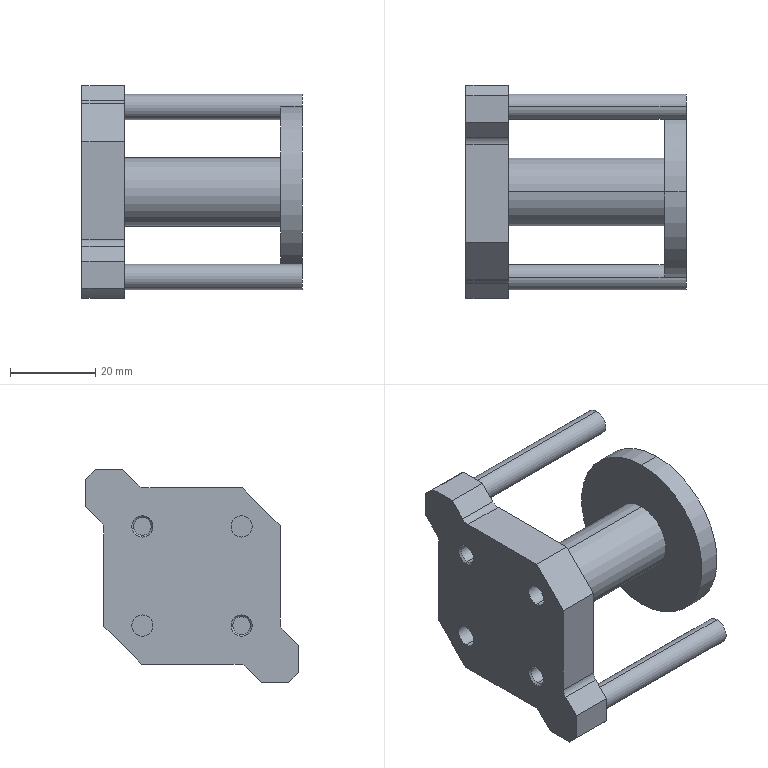Part | STEP file | 1105WWT2_1 | 1 solid | 50 faces | box 51.75 x 50 x 50 mm | volume 33168 mm3 | cylinder 22 | plane 20 | cone 8 | commonest cylinder face diameters 4.134 x4 4.6 x4 5 x4 6 x4 16 x2 40 x2
STEP:
#1=CARTESIAN_POINT('',(-7.,-11.65,9.15));
#2=VERTEX_POINT('',#1);
#3=CARTESIAN_POINT('',(-7.,-11.65,14.15));
#4=VERTEX_POINT('',#3);
#5=CARTESIAN_POINT('',(-7.,-11.65,11.65));
#6=DIRECTION('',(-1.,0.,0.));
#7=DIRECTION('',(0.,0.,1.));
#8=AXIS2_PLACEMENT_3D('',#5,#6,#7);
#9=CIRCLE('',#8,2.5);
#10=EDGE_CURVE('',#2,#4,#9,.T.);
#11=ORIENTED_EDGE('',*,*,#10,.F.);
#12=CARTESIAN_POINT('',(-17.,-11.65,9.15));
#13=VERTEX_POINT('',#12);
#14=CARTESIAN_POINT('',(-17.,-11.65,9.15));
#15=DIRECTION('',(-1.,0.,0.));
#16=VECTOR('',#15,1000.);
#17=LINE('',#14,#16);
#18=EDGE_CURVE('',#2,#13,#17,.T.);
#19=ORIENTED_EDGE('',*,*,#18,.T.);
#20=CARTESIAN_POINT('',(-17.,-11.65,14.15));
#21=VERTEX_POINT('',#20);
#22=CARTESIAN_POINT('',(-17.,-11.65,11.65));
#23=DIRECTION('',(-1.,0.,0.));
#24=DIRECTION('',(0.,0.,1.));
#25=AXIS2_PLACEMENT_3D('',#22,#23,#24);
#26=CIRCLE('',#25,2.5);
#27=EDGE_CURVE('',#13,#21,#26,.T.);
#28=ORIENTED_EDGE('',*,*,#27,.T.);
#29=CARTESIAN_POINT('',(-17.,-11.65,14.15));
#30=DIRECTION('',(-1.,0.,0.));
#31=VECTOR('',#30,1000.);
#32=LINE('',#29,#31);
#33=EDGE_CURVE('',#4,#21,#32,.T.);
#34=ORIENTED_EDGE('',*,*,#33,.F.);
#35=EDGE_LOOP('',(#11,#19,#28,#34));
#36=FACE_OUTER_BOUND('',#35,.T.);
#37=CARTESIAN_POINT('',(-17.,-11.65,11.65));
#38=DIRECTION('',(-1.,0.,0.));
#39=DIRECTION('',(0.,0.,1.));
#40=AXIS2_PLACEMENT_3D('',#37,#38,#39);
#41=CYLINDRICAL_SURFACE('',#40,2.5);
#42=ADVANCED_FACE('',(#36),#41,.F.);
#43=CARTESIAN_POINT('',(-7.,11.65,-14.15));
#44=VERTEX_POINT('',#43);
#45=CARTESIAN_POINT('',(-7.,11.65,-9.15));
#46=VERTEX_POINT('',#45);
#47=CARTESIAN_POINT('',(-7.,11.65,-11.65));
#48=DIRECTION('',(-1.,0.,0.));
#49=DIRECTION('',(0.,0.,1.));
#50=AXIS2_PLACEMENT_3D('',#47,#48,#49);
#51=CIRCLE('',#50,2.5);
#52=EDGE_CURVE('',#44,#46,#51,.T.);
#53=ORIENTED_EDGE('',*,*,#52,.F.);
#54=CARTESIAN_POINT('',(-17.,11.65,-14.15));
#55=VERTEX_POINT('',#54);
#56=CARTESIAN_POINT('',(-17.,11.65,-14.15));
#57=DIRECTION('',(-1.,0.,0.));
#58=VECTOR('',#57,1000.);
#59=LINE('',#56,#58);
#60=EDGE_CURVE('',#44,#55,#59,.T.);
#61=ORIENTED_EDGE('',*,*,#60,.T.);
#62=CARTESIAN_POINT('',(-17.,11.65,-9.15));
#63=VERTEX_POINT('',#62);
#64=CARTESIAN_POINT('',(-17.,11.65,-11.65));
#65=DIRECTION('',(-1.,0.,0.));
#66=DIRECTION('',(0.,0.,1.));
#67=AXIS2_PLACEMENT_3D('',#64,#65,#66);
#68=CIRCLE('',#67,2.5);
#69=EDGE_CURVE('',#55,#63,#68,.T.);
#70=ORIENTED_EDGE('',*,*,#69,.T.);
#71=CARTESIAN_POINT('',(-17.,11.65,-9.15));
#72=DIRECTION('',(-1.,0.,0.));
#73=VECTOR('',#72,1000.);
#74=LINE('',#71,#73);
#75=EDGE_CURVE('',#46,#63,#74,.T.);
#76=ORIENTED_EDGE('',*,*,#75,.F.);
#77=EDGE_LOOP('',(#53,#61,#70,#76));
#78=FACE_OUTER_BOUND('',#77,.T.);
#79=CARTESIAN_POINT('',(-17.,11.65,-11.65));
#80=DIRECTION('',(-1.,0.,0.));
#81=DIRECTION('',(0.,0.,1.));
#82=AXIS2_PLACEMENT_3D('',#79,#80,#81);
#83=CYLINDRICAL_SURFACE('',#82,2.5);
#84=ADVANCED_FACE('',(#78),#83,.F.);
#85=CARTESIAN_POINT('',(-16.567,11.65,9.583));
#86=VERTEX_POINT('',#85);
#87=CARTESIAN_POINT('',(-16.567,11.65,13.717));
#88=VERTEX_POINT('',#87);
#89=CARTESIAN_POINT('',(-16.567,11.65,11.65));
#90=DIRECTION('',(-1.,0.,0.));
#91=DIRECTION('',(0.,1.,0.));
#92=AXIS2_PLACEMENT_3D('',#89,#90,#91);
#93=CIRCLE('',#92,2.067);
#94=EDGE_CURVE('',#86,#88,#93,.T.);
#95=ORIENTED_EDGE('',*,*,#94,.F.);
#96=CARTESIAN_POINT('',(-17.,11.65,9.15));
#97=VERTEX_POINT('',#96);
#98=CARTESIAN_POINT('',(-17.,11.65,9.15));
#99=DIRECTION('',(-0.7071,0.,-0.7071));
#100=VECTOR('',#99,1000.);
#101=LINE('',#98,#100);
#102=EDGE_CURVE('',#86,#97,#101,.T.);
#103=ORIENTED_EDGE('',*,*,#102,.T.);
#104=CARTESIAN_POINT('',(-17.,11.65,14.15));
#105=VERTEX_POINT('',#104);
#106=CARTESIAN_POINT('',(-17.,11.65,11.65));
#107=DIRECTION('',(-1.,0.,0.));
#108=DIRECTION('',(0.,0.,1.));
#109=AXIS2_PLACEMENT_3D('',#106,#107,#108);
#110=CIRCLE('',#109,2.5);
#111=EDGE_CURVE('',#97,#105,#110,.T.);
#112=ORIENTED_EDGE('',*,*,#111,.T.);
#113=CARTESIAN_POINT('',(-17.,11.65,14.15));
#114=DIRECTION('',(-0.7071,0.,0.7071));
#115=VECTOR('',#114,1000.);
#116=LINE('',#113,#115);
#117=EDGE_CURVE('',#88,#105,#116,.T.);
#118=ORIENTED_EDGE('',*,*,#117,.F.);
#119=EDGE_LOOP('',(#95,#103,#112,#118));
#120=FACE_OUTER_BOUND('',#119,.T.);
#121=CARTESIAN_POINT('',(-17.,11.65,11.65));
#122=DIRECTION('',(-1.,0.,0.));
#123=DIRECTION('',(0.,0.,1.));
#124=AXIS2_PLACEMENT_3D('',#121,#122,#123);
#125=CONICAL_SURFACE('',#124,2.5,0.7854);
#126=ADVANCED_FACE('',(#120),#125,.F.);
#127=CARTESIAN_POINT('',(-16.567,-11.65,-13.717));
#128=VERTEX_POINT('',#127);
#129=CARTESIAN_POINT('',(-16.567,-11.65,-9.583));
#130=VERTEX_POINT('',#129);
#131=CARTESIAN_POINT('',(-16.567,-11.65,-11.65));
#132=DIRECTION('',(-1.,0.,0.));
#133=DIRECTION('',(0.,1.,0.));
#134=AXIS2_PLACEMENT_3D('',#131,#132,#133);
#135=CIRCLE('',#134,2.067);
#136=EDGE_CURVE('',#128,#130,#135,.T.);
#137=ORIENTED_EDGE('',*,*,#136,.F.);
#138=CARTESIAN_POINT('',(-17.,-11.65,-14.15));
#139=VERTEX_POINT('',#138);
#140=CARTESIAN_POINT('',(-17.,-11.65,-14.15));
#141=DIRECTION('',(-0.7071,0.,-0.7071));
#142=VECTOR('',#141,1000.);
#143=LINE('',#140,#142);
#144=EDGE_CURVE('',#128,#139,#143,.T.);
#145=ORIENTED_EDGE('',*,*,#144,.T.);
#146=CARTESIAN_POINT('',(-17.,-11.65,-9.15));
#147=VERTEX_POINT('',#146);
#148=CARTESIAN_POINT('',(-17.,-11.65,-11.65));
#149=DIRECTION('',(-1.,0.,0.));
#150=DIRECTION('',(0.,0.,1.));
#151=AXIS2_PLACEMENT_3D('',#148,#149,#150);
#152=CIRCLE('',#151,2.5);
#153=EDGE_CURVE('',#139,#147,#152,.T.);
#154=ORIENTED_EDGE('',*,*,#153,.T.);
#155=CARTESIAN_POINT('',(-17.,-11.65,-9.15));
#156=DIRECTION('',(-0.7071,0.,0.7071));
#157=VECTOR('',#156,1000.);
#158=LINE('',#155,#157);
#159=EDGE_CURVE('',#130,#147,#158,.T.);
#160=ORIENTED_EDGE('',*,*,#159,.F.);
#161=EDGE_LOOP('',(#137,#145,#154,#160));
#162=FACE_OUTER_BOUND('',#161,.T.);
#163=CARTESIAN_POINT('',(-17.,-11.65,-11.65));
#164=DIRECTION('',(-1.,0.,0.));
#165=DIRECTION('',(0.,0.,1.));
#166=AXIS2_PLACEMENT_3D('',#163,#164,#165);
#167=CONICAL_SURFACE('',#166,2.5,0.7854);
#168=ADVANCED_FACE('',(#162),#167,.F.);
#169=ORIENTED_EDGE('',*,*,#94,.T.);
#170=CARTESIAN_POINT('',(-7.433,11.65,13.717));
#171=VERTEX_POINT('',#170);
#172=CARTESIAN_POINT('',(-12.,11.65,13.717));
#173=DIRECTION('',(1.,0.,0.));
#174=VECTOR('',#173,1000.);
#175=LINE('',#172,#174);
#176=EDGE_CURVE('',#88,#171,#175,.T.);
#177=ORIENTED_EDGE('',*,*,#176,.T.);
#178=CARTESIAN_POINT('',(-7.433,11.65,9.583));
#179=VERTEX_POINT('',#178);
#180=CARTESIAN_POINT('',(-7.433,11.65,11.65));
#181=DIRECTION('',(-1.,0.,0.));
#182=DIRECTION('',(0.,0.,-1.));
#183=AXIS2_PLACEMENT_3D('',#180,#181,#182);
#184=CIRCLE('',#183,2.067);
#185=EDGE_CURVE('',#179,#171,#184,.T.);
#186=ORIENTED_EDGE('',*,*,#185,.F.);
#187=CARTESIAN_POINT('',(-12.,11.65,9.583));
#188=DIRECTION('',(1.,0.,0.));
#189=VECTOR('',#188,1000.);
#190=LINE('',#187,#189);
#191=EDGE_CURVE('',#86,#179,#190,.T.);
#192=ORIENTED_EDGE('',*,*,#191,.F.);
#193=EDGE_LOOP('',(#169,#177,#186,#192));
#194=FACE_OUTER_BOUND('',#193,.T.);
#195=CARTESIAN_POINT('',(-12.,11.65,11.65));
#196=DIRECTION('',(1.,0.,0.));
#197=DIRECTION('',(0.,0.,-1.));
#198=AXIS2_PLACEMENT_3D('',#195,#196,#197);
#199=CYLINDRICAL_SURFACE('',#198,2.067);
#200=ADVANCED_FACE('',(#194),#199,.F.);
#201=ORIENTED_EDGE('',*,*,#136,.T.);
#202=CARTESIAN_POINT('',(-7.433,-11.65,-9.583));
#203=VERTEX_POINT('',#202);
#204=CARTESIAN_POINT('',(-12.,-11.65,-9.583));
#205=DIRECTION('',(1.,0.,0.));
#206=VECTOR('',#205,1000.);
#207=LINE('',#204,#206);
#208=EDGE_CURVE('',#130,#203,#207,.T.);
#209=ORIENTED_EDGE('',*,*,#208,.T.);
#210=CARTESIAN_POINT('',(-7.433,-11.65,-13.717));
#211=VERTEX_POINT('',#210);
#212=CARTESIAN_POINT('',(-7.433,-11.65,-11.65));
#213=DIRECTION('',(-1.,0.,0.));
#214=DIRECTION('',(0.,0.,-1.));
#215=AXIS2_PLACEMENT_3D('',#212,#213,#214);
#216=CIRCLE('',#215,2.067);
#217=EDGE_CURVE('',#211,#203,#216,.T.);
#218=ORIENTED_EDGE('',*,*,#217,.F.);
#219=CARTESIAN_POINT('',(-12.,-11.65,-13.717));
#220=DIRECTION('',(1.,0.,0.));
#221=VECTOR('',#220,1000.);
#222=LINE('',#219,#221);
#223=EDGE_CURVE('',#128,#211,#222,.T.);
#224=ORIENTED_EDGE('',*,*,#223,.F.);
#225=EDGE_LOOP('',(#201,#209,#218,#224));
#226=FACE_OUTER_BOUND('',#225,.T.);
#227=CARTESIAN_POINT('',(-12.,-11.65,-11.65));
#228=DIRECTION('',(1.,0.,0.));
#229=DIRECTION('',(0.,0.,-1.));
#230=AXIS2_PLACEMENT_3D('',#227,#228,#229);
#231=CYLINDRICAL_SURFACE('',#230,2.067);
#232=ADVANCED_FACE('',(#226),#231,.F.);
#233=ORIENTED_EDGE('',*,*,#185,.T.);
#234=CARTESIAN_POINT('',(-7.,11.65,14.15));
#235=VERTEX_POINT('',#234);
#236=CARTESIAN_POINT('',(-7.,11.65,14.15));
#237=DIRECTION('',(0.7071,0.,0.7071));
#238=VECTOR('',#237,1000.);
#239=LINE('',#236,#238);
#240=EDGE_CURVE('',#171,#235,#239,.T.);
#241=ORIENTED_EDGE('',*,*,#240,.T.);
#242=CARTESIAN_POINT('',(-7.,11.65,9.15));
#243=VERTEX_POINT('',#242);
#244=CARTESIAN_POINT('',(-7.,11.65,11.65));
#245=DIRECTION('',(-1.,0.,0.));
#246=DIRECTION('',(0.,0.,-1.));
#247=AXIS2_PLACEMENT_3D('',#244,#245,#246);
#248=CIRCLE('',#247,2.5);
#249=EDGE_CURVE('',#243,#235,#248,.T.);
#250=ORIENTED_EDGE('',*,*,#249,.F.);
#251=CARTESIAN_POINT('',(-7.,11.65,9.15));
#252=DIRECTION('',(0.7071,0.,-0.7071));
#253=VECTOR('',#252,1000.);
#254=LINE('',#251,#253);
#255=EDGE_CURVE('',#179,#243,#254,.T.);
#256=ORIENTED_EDGE('',*,*,#255,.F.);
#257=EDGE_LOOP('',(#233,#241,#250,#256));
#258=FACE_OUTER_BOUND('',#257,.T.);
#259=CARTESIAN_POINT('',(-7.,11.65,11.65));
#260=DIRECTION('',(1.,0.,0.));
#261=DIRECTION('',(0.,0.,-1.));
#262=AXIS2_PLACEMENT_3D('',#259,#260,#261);
#263=CONICAL_SURFACE('',#262,2.5,0.7854);
#264=ADVANCED_FACE('',(#258),#263,.F.);
#265=ORIENTED_EDGE('',*,*,#217,.T.);
#266=CARTESIAN_POINT('',(-7.,-11.65,-9.15));
#267=VERTEX_POINT('',#266);
#268=CARTESIAN_POINT('',(-7.,-11.65,-9.15));
#269=DIRECTION('',(0.7071,0.,0.7071));
#270=VECTOR('',#269,1000.);
#271=LINE('',#268,#270);
#272=EDGE_CURVE('',#203,#267,#271,.T.);
#273=ORIENTED_EDGE('',*,*,#272,.T.);
#274=CARTESIAN_POINT('',(-7.,-11.65,-14.15));
#275=VERTEX_POINT('',#274);
#276=CARTESIAN_POINT('',(-7.,-11.65,-11.65));
#277=DIRECTION('',(-1.,0.,0.));
#278=DIRECTION('',(0.,0.,-1.));
#279=AXIS2_PLACEMENT_3D('',#276,#277,#278);
#280=CIRCLE('',#279,2.5);
#281=EDGE_CURVE('',#275,#267,#280,.T.);
#282=ORIENTED_EDGE('',*,*,#281,.F.);
#283=CARTESIAN_POINT('',(-7.,-11.65,-14.15));
#284=DIRECTION('',(0.7071,0.,-0.7071));
#285=VECTOR('',#284,1000.);
#286=LINE('',#283,#285);
#287=EDGE_CURVE('',#211,#275,#286,.T.);
#288=ORIENTED_EDGE('',*,*,#287,.F.);
#289=EDGE_LOOP('',(#265,#273,#282,#288));
#290=FACE_OUTER_BOUND('',#289,.T.);
#291=CARTESIAN_POINT('',(-7.,-11.65,-11.65));
#292=DIRECTION('',(1.,0.,0.));
#293=DIRECTION('',(0.,0.,-1.));
#294=AXIS2_PLACEMENT_3D('',#291,#292,#293);
#295=CONICAL_SURFACE('',#294,2.5,0.7854);
#296=ADVANCED_FACE('',(#290),#295,.F.);
#297=CARTESIAN_POINT('',(-7.,0.,8.));
#298=VERTEX_POINT('',#297);
#299=CARTESIAN_POINT('',(-7.,0.,-8.));
#300=VERTEX_POINT('',#299);
#301=CARTESIAN_POINT('',(-7.,0.,0.));
#302=DIRECTION('',(-1.,0.,0.));
#303=DIRECTION('',(0.,0.,-1.));
#304=AXIS2_PLACEMENT_3D('',#301,#302,#303);
#305=CIRCLE('',#304,8.);
#306=EDGE_CURVE('',#298,#300,#305,.T.);
#307=ORIENTED_EDGE('',*,*,#306,.F.);
#308=CARTESIAN_POINT('',(29.75,0.,8.));
#309=VERTEX_POINT('',#308);
#310=CARTESIAN_POINT('',(11.375,0.,8.));
#311=DIRECTION('',(1.,0.,0.));
#312=VECTOR('',#311,1000.);
#313=LINE('',#310,#312);
#314=EDGE_CURVE('',#298,#309,#313,.T.);
#315=ORIENTED_EDGE('',*,*,#314,.T.);
#316=CARTESIAN_POINT('',(29.75,0.,-8.));
#317=VERTEX_POINT('',#316);
#318=CARTESIAN_POINT('',(29.75,0.,0.));
#319=DIRECTION('',(-1.,0.,0.));
#320=DIRECTION('',(0.,0.,-1.));
#321=AXIS2_PLACEMENT_3D('',#318,#319,#320);
#322=CIRCLE('',#321,8.);
#323=EDGE_CURVE('',#309,#317,#322,.T.);
#324=ORIENTED_EDGE('',*,*,#323,.T.);
#325=CARTESIAN_POINT('',(11.375,0.,-8.));
#326=DIRECTION('',(1.,0.,0.));
#327=VECTOR('',#326,1000.);
#328=LINE('',#325,#327);
#329=EDGE_CURVE('',#300,#317,#328,.T.);
#330=ORIENTED_EDGE('',*,*,#329,.F.);
#331=EDGE_LOOP('',(#307,#315,#324,#330));
#332=FACE_OUTER_BOUND('',#331,.T.);
#333=CARTESIAN_POINT('',(11.375,0.,0.));
#334=DIRECTION('',(1.,0.,0.));
#335=DIRECTION('',(0.,0.,-1.));
#336=AXIS2_PLACEMENT_3D('',#333,#334,#335);
#337=CYLINDRICAL_SURFACE('',#336,8.);
#338=ADVANCED_FACE('',(#332),#337,.T.);
#339=CARTESIAN_POINT('',(-7.,20.,23.));
#340=VERTEX_POINT('',#339);
#341=CARTESIAN_POINT('',(-7.,20.,17.));
#342=VERTEX_POINT('',#341);
#343=CARTESIAN_POINT('',(-7.,20.,20.));
#344=DIRECTION('',(-1.,0.,0.));
#345=DIRECTION('',(0.,0.,-1.));
#346=AXIS2_PLACEMENT_3D('',#343,#344,#345);
#347=CIRCLE('',#346,3.);
#348=EDGE_CURVE('',#340,#342,#347,.T.);
#349=ORIENTED_EDGE('',*,*,#348,.F.);
#350=CARTESIAN_POINT('',(34.75,20.,23.));
#351=VERTEX_POINT('',#350);
#352=CARTESIAN_POINT('',(13.875,20.,23.));
#353=DIRECTION('',(1.,0.,0.));
#354=VECTOR('',#353,1000.);
#355=LINE('',#352,#354);
#356=EDGE_CURVE('',#340,#351,#355,.T.);
#357=ORIENTED_EDGE('',*,*,#356,.T.);
#358=CARTESIAN_POINT('',(34.75,20.,17.));
#359=VERTEX_POINT('',#358);
#360=CARTESIAN_POINT('',(34.75,20.,20.));
#361=DIRECTION('',(-1.,0.,0.));
#362=DIRECTION('',(0.,0.,-1.));
#363=AXIS2_PLACEMENT_3D('',#360,#361,#362);
#364=CIRCLE('',#363,3.);
#365=EDGE_CURVE('',#351,#359,#364,.T.);
#366=ORIENTED_EDGE('',*,*,#365,.T.);
#367=CARTESIAN_POINT('',(13.875,20.,17.));
#368=DIRECTION('',(1.,0.,0.));
#369=VECTOR('',#368,1000.);
#370=LINE('',#367,#369);
#371=EDGE_CURVE('',#342,#359,#370,.T.);
#372=ORIENTED_EDGE('',*,*,#371,.F.);
#373=EDGE_LOOP('',(#349,#357,#366,#372));
#374=FACE_OUTER_BOUND('',#373,.T.);
#375=CARTESIAN_POINT('',(13.875,20.,20.));
#376=DIRECTION('',(1.,0.,0.));
#377=DIRECTION('',(0.,0.,-1.));
#378=AXIS2_PLACEMENT_3D('',#375,#376,#377);
#379=CYLINDRICAL_SURFACE('',#378,3.);
#380=ADVANCED_FACE('',(#374),#379,.T.);
#381=CARTESIAN_POINT('',(-7.,-20.,-17.));
#382=VERTEX_POINT('',#381);
#383=CARTESIAN_POINT('',(-7.,-20.,-23.));
#384=VERTEX_POINT('',#383);
#385=CARTESIAN_POINT('',(-7.,-20.,-20.));
#386=DIRECTION('',(-1.,0.,0.));
#387=DIRECTION('',(0.,0.,-1.));
#388=AXIS2_PLACEMENT_3D('',#385,#386,#387);
#389=CIRCLE('',#388,3.);
#390=EDGE_CURVE('',#382,#384,#389,.T.);
#391=ORIENTED_EDGE('',*,*,#390,.F.);
#392=CARTESIAN_POINT('',(34.75,-20.,-17.));
#393=VERTEX_POINT('',#392);
#394=CARTESIAN_POINT('',(13.875,-20.,-17.));
#395=DIRECTION('',(1.,0.,0.));
#396=VECTOR('',#395,1000.);
#397=LINE('',#394,#396);
#398=EDGE_CURVE('',#382,#393,#397,.T.);
#399=ORIENTED_EDGE('',*,*,#398,.T.);
#400=CARTESIAN_POINT('',(34.75,-20.,-23.));
#401=VERTEX_POINT('',#400);
#402=CARTESIAN_POINT('',(34.75,-20.,-20.));
#403=DIRECTION('',(-1.,0.,0.));
#404=DIRECTION('',(0.,0.,-1.));
#405=AXIS2_PLACEMENT_3D('',#402,#403,#404);
#406=CIRCLE('',#405,3.);
#407=EDGE_CURVE('',#393,#401,#406,.T.);
#408=ORIENTED_EDGE('',*,*,#407,.T.);
#409=CARTESIAN_POINT('',(13.875,-20.,-23.));
#410=DIRECTION('',(1.,0.,0.));
#411=VECTOR('',#410,1000.);
#412=LINE('',#409,#411);
#413=EDGE_CURVE('',#384,#401,#412,.T.);
#414=ORIENTED_EDGE('',*,*,#413,.F.);
#415=EDGE_LOOP('',(#391,#399,#408,#414));
#416=FACE_OUTER_BOUND('',#415,.T.);
#417=CARTESIAN_POINT('',(13.875,-20.,-20.));
#418=DIRECTION('',(1.,0.,0.));
#419=DIRECTION('',(0.,0.,-1.));
#420=AXIS2_PLACEMENT_3D('',#417,#418,#419);
#421=CYLINDRICAL_SURFACE('',#420,3.);
#422=ADVANCED_FACE('',(#416),#421,.T.);
#423=CARTESIAN_POINT('',(29.75,0.,20.));
#424=VERTEX_POINT('',#423);
#425=CARTESIAN_POINT('',(29.75,0.,-20.));
#426=VERTEX_POINT('',#425);
#427=CARTESIAN_POINT('',(29.75,0.,0.));
#428=DIRECTION('',(-1.,0.,0.));
#429=DIRECTION('',(0.,0.,-1.));
#430=AXIS2_PLACEMENT_3D('',#427,#428,#429);
#431=CIRCLE('',#430,20.);
#432=EDGE_CURVE('',#424,#426,#431,.T.);
#433=ORIENTED_EDGE('',*,*,#432,.F.);
#434=CARTESIAN_POINT('',(34.75,0.,20.));
#435=VERTEX_POINT('',#434);
#436=CARTESIAN_POINT('',(32.25,0.,20.));
#437=DIRECTION('',(1.,0.,0.));
#438=VECTOR('',#437,1000.);
#439=LINE('',#436,#438);
#440=EDGE_CURVE('',#424,#435,#439,.T.);
#441=ORIENTED_EDGE('',*,*,#440,.T.);
#442=CARTESIAN_POINT('',(34.75,0.,-20.));
#443=VERTEX_POINT('',#442);
#444=CARTESIAN_POINT('',(34.75,0.,0.));
#445=DIRECTION('',(-1.,0.,0.));
#446=DIRECTION('',(0.,0.,-1.));
#447=AXIS2_PLACEMENT_3D('',#444,#445,#446);
#448=CIRCLE('',#447,20.);
#449=EDGE_CURVE('',#435,#443,#448,.T.);
#450=ORIENTED_EDGE('',*,*,#449,.T.);
#451=CARTESIAN_POINT('',(32.25,0.,-20.));
#452=DIRECTION('',(1.,0.,0.));
#453=VECTOR('',#452,1000.);
#454=LINE('',#451,#453);
#455=EDGE_CURVE('',#426,#443,#454,.T.);
#456=ORIENTED_EDGE('',*,*,#455,.F.);
#457=EDGE_LOOP('',(#433,#441,#450,#456));
#458=FACE_OUTER_BOUND('',#457,.T.);
#459=CARTESIAN_POINT('',(32.25,0.,0.));
#460=DIRECTION('',(1.,0.,0.));
#461=DIRECTION('',(0.,0.,-1.));
#462=AXIS2_PLACEMENT_3D('',#459,#460,#461);
#463=CYLINDRICAL_SURFACE('',#462,20.);
#464=ADVANCED_FACE('',(#458),#463,.T.);
#465=CARTESIAN_POINT('',(-17.,-11.65,11.65));
#466=DIRECTION('',(-1.,0.,0.));
#467=DIRECTION('',(0.,0.,1.));
#468=AXIS2_PLACEMENT_3D('',#465,#466,#467);
#469=CIRCLE('',#468,2.5);
#470=EDGE_CURVE('',#21,#13,#469,.T.);
#471=ORIENTED_EDGE('',*,*,#470,.F.);
#472=ORIENTED_EDGE('',*,*,#27,.F.);
#473=EDGE_LOOP('',(#471,#472));
#474=FACE_BOUND('',#473,.T.);
#475=CARTESIAN_POINT('',(-17.,11.65,-11.65));
#476=DIRECTION('',(-1.,0.,0.));
#477=DIRECTION('',(0.,0.,1.));
#478=AXIS2_PLACEMENT_3D('',#475,#476,#477);
#479=CIRCLE('',#478,2.5);
#480=EDGE_CURVE('',#63,#55,#479,.T.);
#481=ORIENTED_EDGE('',*,*,#480,.F.);
#482=ORIENTED_EDGE('',*,*,#69,.F.);
#483=EDGE_LOOP('',(#481,#482));
#484=FACE_BOUND('',#483,.T.);
#485=CARTESIAN_POINT('',(-17.,22.673,25.));
#486=VERTEX_POINT('',#485);
#487=CARTESIAN_POINT('',(-17.,16.3,25.));
#488=VERTEX_POINT('',#487);
#489=CARTESIAN_POINT('',(-17.,0.,25.));
#490=DIRECTION('',(0.,-1.,0.));
#491=VECTOR('',#490,1000.);
#492=LINE('',#489,#491);
#493=EDGE_CURVE('',#486,#488,#492,.T.);
#494=ORIENTED_EDGE('',*,*,#493,.F.);
#495=CARTESIAN_POINT('',(-17.,25.,22.673));
#496=VERTEX_POINT('',#495);
#497=CARTESIAN_POINT('',(-17.,0.,0.));
#498=DIRECTION('',(1.,0.,0.));
#499=DIRECTION('',(0.,0.,1.));
#500=AXIS2_PLACEMENT_3D('',#497,#498,#499);
#501=CIRCLE('',#500,33.75);
#502=EDGE_CURVE('',#496,#486,#501,.T.);
#503=ORIENTED_EDGE('',*,*,#502,.F.);
#504=CARTESIAN_POINT('',(-17.,25.,16.3));
#505=VERTEX_POINT('',#504);
#506=CARTESIAN_POINT('',(-17.,25.,0.));
#507=DIRECTION('',(0.,0.,1.));
#508=VECTOR('',#507,1000.);
#509=LINE('',#506,#508);
#510=EDGE_CURVE('',#505,#496,#509,.T.);
#511=ORIENTED_EDGE('',*,*,#510,.F.);
#512=CARTESIAN_POINT('',(-17.,21.441,12.741));
#513=VERTEX_POINT('',#512);
#514=CARTESIAN_POINT('',(-17.,21.441,12.741));
#515=DIRECTION('',(0.,0.7071,0.7071));
#516=VECTOR('',#515,1000.);
#517=LINE('',#514,#516);
#518=EDGE_CURVE('',#513,#505,#517,.T.);
#519=ORIENTED_EDGE('',*,*,#518,.F.);
#520=CARTESIAN_POINT('',(-17.,20.7,11.05));
#521=VERTEX_POINT('',#520);
#522=CARTESIAN_POINT('',(-17.,23.,11.05));
#523=DIRECTION('',(-1.,0.,0.));
#524=DIRECTION('',(0.,0.,1.));
#525=AXIS2_PLACEMENT_3D('',#522,#523,#524);
#526=CIRCLE('',#525,2.3);
#527=EDGE_CURVE('',#521,#513,#526,.T.);
#528=ORIENTED_EDGE('',*,*,#527,.F.);
#529=CARTESIAN_POINT('',(-17.,20.7,-11.827));
#530=VERTEX_POINT('',#529);
#531=CARTESIAN_POINT('',(-17.,20.7,0.));
#532=DIRECTION('',(0.,0.,1.));
#533=VECTOR('',#532,1000.);
#534=LINE('',#531,#533);
#535=EDGE_CURVE('',#530,#521,#534,.T.);
#536=ORIENTED_EDGE('',*,*,#535,.F.);
#537=CARTESIAN_POINT('',(-17.,11.827,-20.7));
#538=VERTEX_POINT('',#537);
#539=CARTESIAN_POINT('',(-17.,11.827,-20.7));
#540=DIRECTION('',(0.,0.7071,0.7071));
#541=VECTOR('',#540,1000.);
#542=LINE('',#539,#541);
#543=EDGE_CURVE('',#538,#530,#542,.T.);
#544=ORIENTED_EDGE('',*,*,#543,.F.);
#545=CARTESIAN_POINT('',(-17.,-11.05,-20.7));
#546=VERTEX_POINT('',#545);
#547=CARTESIAN_POINT('',(-17.,0.,-20.7));
#548=DIRECTION('',(0.,1.,0.));
#549=VECTOR('',#548,1000.);
#550=LINE('',#547,#549);
#551=EDGE_CURVE('',#546,#538,#550,.T.);
#552=ORIENTED_EDGE('',*,*,#551,.F.);
#553=CARTESIAN_POINT('',(-17.,-12.741,-21.441));
#554=VERTEX_POINT('',#553);
#555=CARTESIAN_POINT('',(-17.,-11.05,-23.));
#556=DIRECTION('',(-1.,0.,0.));
#557=DIRECTION('',(0.,0.,1.));
#558=AXIS2_PLACEMENT_3D('',#555,#556,#557);
#559=CIRCLE('',#558,2.3);
#560=EDGE_CURVE('',#554,#546,#559,.T.);
#561=ORIENTED_EDGE('',*,*,#560,.F.);
#562=CARTESIAN_POINT('',(-17.,-16.3,-25.));
#563=VERTEX_POINT('',#562);
#564=CARTESIAN_POINT('',(-17.,-16.3,-25.));
#565=DIRECTION('',(0.,0.7071,0.7071));
#566=VECTOR('',#565,1000.);
#567=LINE('',#564,#566);
#568=EDGE_CURVE('',#563,#554,#567,.T.);
#569=ORIENTED_EDGE('',*,*,#568,.F.);
#570=CARTESIAN_POINT('',(-17.,-22.673,-25.));
#571=VERTEX_POINT('',#570);
#572=CARTESIAN_POINT('',(-17.,0.,-25.));
#573=DIRECTION('',(0.,1.,0.));
#574=VECTOR('',#573,1000.);
#575=LINE('',#572,#574);
#576=EDGE_CURVE('',#571,#563,#575,.T.);
#577=ORIENTED_EDGE('',*,*,#576,.F.);
#578=CARTESIAN_POINT('',(-17.,-25.,-22.673));
#579=VERTEX_POINT('',#578);
#580=CARTESIAN_POINT('',(-17.,0.,0.));
#581=DIRECTION('',(1.,0.,0.));
#582=DIRECTION('',(0.,0.,1.));
#583=AXIS2_PLACEMENT_3D('',#580,#581,#582);
#584=CIRCLE('',#583,33.75);
#585=EDGE_CURVE('',#579,#571,#584,.T.);
#586=ORIENTED_EDGE('',*,*,#585,.F.);
#587=CARTESIAN_POINT('',(-17.,-25.,-16.3));
#588=VERTEX_POINT('',#587);
#589=CARTESIAN_POINT('',(-17.,-25.,0.));
#590=DIRECTION('',(0.,0.,-1.));
#591=VECTOR('',#590,1000.);
#592=LINE('',#589,#591);
#593=EDGE_CURVE('',#588,#579,#592,.T.);
#594=ORIENTED_EDGE('',*,*,#593,.F.);
#595=CARTESIAN_POINT('',(-17.,-21.441,-12.741));
#596=VERTEX_POINT('',#595);
#597=CARTESIAN_POINT('',(-17.,-21.441,-12.741));
#598=DIRECTION('',(0.,-0.7071,-0.7071));
#599=VECTOR('',#598,1000.);
#600=LINE('',#597,#599);
#601=EDGE_CURVE('',#596,#588,#600,.T.);
#602=ORIENTED_EDGE('',*,*,#601,.F.);
#603=CARTESIAN_POINT('',(-17.,-20.7,-11.05));
#604=VERTEX_POINT('',#603);
#605=CARTESIAN_POINT('',(-17.,-23.,-11.05));
#606=DIRECTION('',(-1.,0.,0.));
#607=DIRECTION('',(0.,0.,1.));
#608=AXIS2_PLACEMENT_3D('',#605,#606,#607);
#609=CIRCLE('',#608,2.3);
#610=EDGE_CURVE('',#604,#596,#609,.T.);
#611=ORIENTED_EDGE('',*,*,#610,.F.);
#612=CARTESIAN_POINT('',(-17.,-20.7,11.827));
#613=VERTEX_POINT('',#612);
#614=CARTESIAN_POINT('',(-17.,-20.7,0.));
#615=DIRECTION('',(0.,0.,-1.));
#616=VECTOR('',#615,1000.);
#617=LINE('',#614,#616);
#618=EDGE_CURVE('',#613,#604,#617,.T.);
#619=ORIENTED_EDGE('',*,*,#618,.F.);
#620=CARTESIAN_POINT('',(-17.,-11.827,20.7));
#621=VERTEX_POINT('',#620);
#622=CARTESIAN_POINT('',(-17.,-11.827,20.7));
#623=DIRECTION('',(0.,-0.7071,-0.7071));
#624=VECTOR('',#623,1000.);
#625=LINE('',#622,#624);
#626=EDGE_CURVE('',#621,#613,#625,.T.);
#627=ORIENTED_EDGE('',*,*,#626,.F.);
#628=CARTESIAN_POINT('',(-17.,11.05,20.7));
#629=VERTEX_POINT('',#628);
#630=CARTESIAN_POINT('',(-17.,0.,20.7));
#631=DIRECTION('',(0.,-1.,0.));
#632=VECTOR('',#631,1000.);
#633=LINE('',#630,#632);
#634=EDGE_CURVE('',#629,#621,#633,.T.);
#635=ORIENTED_EDGE('',*,*,#634,.F.);
#636=CARTESIAN_POINT('',(-17.,12.741,21.441));
#637=VERTEX_POINT('',#636);
#638=CARTESIAN_POINT('',(-17.,11.05,23.));
#639=DIRECTION('',(-1.,0.,0.));
#640=DIRECTION('',(0.,0.,1.));
#641=AXIS2_PLACEMENT_3D('',#638,#639,#640);
#642=CIRCLE('',#641,2.3);
#643=EDGE_CURVE('',#637,#629,#642,.T.);
#644=ORIENTED_EDGE('',*,*,#643,.F.);
#645=CARTESIAN_POINT('',(-17.,16.3,25.));
#646=DIRECTION('',(0.,-0.7071,-0.7071));
#647=VECTOR('',#646,1000.);
#648=LINE('',#645,#647);
#649=EDGE_CURVE('',#488,#637,#648,.T.);
#650=ORIENTED_EDGE('',*,*,#649,.F.);
#651=EDGE_LOOP('',(#494,#503,#511,#519,#528,#536,#544,#552,#561,#569,#577,#586,#594,#602,#611,#619,#627,#635,#644,#650));
#652=FACE_OUTER_BOUND('',#651,.T.);
#653=CARTESIAN_POINT('',(-17.,11.65,11.65));
#654=DIRECTION('',(-1.,0.,0.));
#655=DIRECTION('',(0.,0.,1.));
#656=AXIS2_PLACEMENT_3D('',#653,#654,#655);
#657=CIRCLE('',#656,2.5);
#658=EDGE_CURVE('',#105,#97,#657,.T.);
#659=ORIENTED_EDGE('',*,*,#658,.F.);
#660=ORIENTED_EDGE('',*,*,#111,.F.);
#661=EDGE_LOOP('',(#659,#660));
#662=FACE_BOUND('',#661,.T.);
#663=CARTESIAN_POINT('',(-17.,-11.65,-11.65));
#664=DIRECTION('',(-1.,0.,0.));
#665=DIRECTION('',(0.,0.,1.));
#666=AXIS2_PLACEMENT_3D('',#663,#664,#665);
#667=CIRCLE('',#666,2.5);
#668=EDGE_CURVE('',#147,#139,#667,.T.);
#669=ORIENTED_EDGE('',*,*,#668,.F.);
#670=ORIENTED_EDGE('',*,*,#153,.F.);
#671=EDGE_LOOP('',(#669,#670));
#672=FACE_BOUND('',#671,.T.);
#673=CARTESIAN_POINT('',(-17.,0.,0.));
#674=DIRECTION('',(1.,0.,0.));
#675=DIRECTION('',(0.,0.,-1.));
#676=AXIS2_PLACEMENT_3D('',#673,#674,#675);
#677=PLANE('',#676);
#678=ADVANCED_FACE('',(#474,#484,#652,#662,#672),#677,.F.);
#679=ORIENTED_EDGE('',*,*,#18,.F.);
#680=CARTESIAN_POINT('',(-7.,-11.65,11.65));
#681=DIRECTION('',(-1.,0.,0.));
#682=DIRECTION('',(0.,0.,1.));
#683=AXIS2_PLACEMENT_3D('',#680,#681,#682);
#684=CIRCLE('',#683,2.5);
#685=EDGE_CURVE('',#4,#2,#684,.T.);
#686=ORIENTED_EDGE('',*,*,#685,.F.);
#687=ORIENTED_EDGE('',*,*,#33,.T.);
#688=ORIENTED_EDGE('',*,*,#470,.T.);
#689=EDGE_LOOP('',(#679,#686,#687,#688));
#690=FACE_OUTER_BOUND('',#689,.T.);
#691=CARTESIAN_POINT('',(-17.,-11.65,11.65));
#692=DIRECTION('',(-1.,0.,0.));
#693=DIRECTION('',(0.,0.,1.));
#694=AXIS2_PLACEMENT_3D('',#691,#692,#693);
#695=CYLINDRICAL_SURFACE('',#694,2.5);
#696=ADVANCED_FACE('',(#690),#695,.F.);
#697=ORIENTED_EDGE('',*,*,#60,.F.);
#698=CARTESIAN_POINT('',(-7.,11.65,-11.65));
#699=DIRECTION('',(-1.,0.,0.));
#700=DIRECTION('',(0.,0.,1.));
#701=AXIS2_PLACEMENT_3D('',#698,#699,#700);
#702=CIRCLE('',#701,2.5);
#703=EDGE_CURVE('',#46,#44,#702,.T.);
#704=ORIENTED_EDGE('',*,*,#703,.F.);
#705=ORIENTED_EDGE('',*,*,#75,.T.);
#706=ORIENTED_EDGE('',*,*,#480,.T.);
#707=EDGE_LOOP('',(#697,#704,#705,#706));
#708=FACE_OUTER_BOUND('',#707,.T.);
#709=CARTESIAN_POINT('',(-17.,11.65,-11.65));
#710=DIRECTION('',(-1.,0.,0.));
#711=DIRECTION('',(0.,0.,1.));
#712=AXIS2_PLACEMENT_3D('',#709,#710,#711);
#713=CYLINDRICAL_SURFACE('',#712,2.5);
#714=ADVANCED_FACE('',(#708),#713,.F.);
#715=ORIENTED_EDGE('',*,*,#649,.T.);
#716=CARTESIAN_POINT('',(-7.,12.741,21.441));
#717=VERTEX_POINT('',#716);
#718=CARTESIAN_POINT('',(-17.,12.741,21.441));
#719=DIRECTION('',(1.,0.,0.));
#720=VECTOR('',#719,1000.);
#721=LINE('',#718,#720);
#722=EDGE_CURVE('',#637,#717,#721,.T.);
#723=ORIENTED_EDGE('',*,*,#722,.T.);
#724=CARTESIAN_POINT('',(-7.,16.3,25.));
#725=VERTEX_POINT('',#724);
#726=CARTESIAN_POINT('',(-7.,12.741,21.441));
#727=DIRECTION('',(0.,0.7071,0.7071));
#728=VECTOR('',#727,1000.);
#729=LINE('',#726,#728);
#730=EDGE_CURVE('',#717,#725,#729,.T.);
#731=ORIENTED_EDGE('',*,*,#730,.T.);
#732=CARTESIAN_POINT('',(-17.,16.3,25.));
#733=DIRECTION('',(-1.,0.,0.));
#734=VECTOR('',#733,1000.);
#735=LINE('',#732,#734);
#736=EDGE_CURVE('',#725,#488,#735,.T.);
#737=ORIENTED_EDGE('',*,*,#736,.T.);
#738=EDGE_LOOP('',(#715,#723,#731,#737));
#739=FACE_OUTER_BOUND('',#738,.T.);
#740=CARTESIAN_POINT('',(-17.,12.741,21.441));
#741=DIRECTION('',(0.,-0.7071,0.7071));
#742=DIRECTION('',(0.,-0.7071,-0.7071));
#743=AXIS2_PLACEMENT_3D('',#740,#741,#742);
#744=PLANE('',#743);
#745=ADVANCED_FACE('',(#739),#744,.T.);
#746=ORIENTED_EDGE('',*,*,#493,.T.);
#747=ORIENTED_EDGE('',*,*,#736,.F.);
#748=CARTESIAN_POINT('',(-7.,22.673,25.));
#749=VERTEX_POINT('',#748);
#750=CARTESIAN_POINT('',(-7.,16.3,25.));
#751=DIRECTION('',(0.,1.,0.));
#752=VECTOR('',#751,1000.);
#753=LINE('',#750,#752);
#754=EDGE_CURVE('',#725,#749,#753,.T.);
#755=ORIENTED_EDGE('',*,*,#754,.T.);
#756=CARTESIAN_POINT('',(-17.,22.673,25.));
#757=DIRECTION('',(-1.,0.,0.));
#758=VECTOR('',#757,1000.);
#759=LINE('',#756,#758);
#760=EDGE_CURVE('',#749,#486,#759,.T.);
#761=ORIENTED_EDGE('',*,*,#760,.T.);
#762=EDGE_LOOP('',(#746,#747,#755,#761));
#763=FACE_OUTER_BOUND('',#762,.T.);
#764=CARTESIAN_POINT('',(-17.,16.3,25.));
#765=DIRECTION('',(0.,0.,1.));
#766=DIRECTION('',(1.,0.,0.));
#767=AXIS2_PLACEMENT_3D('',#764,#765,#766);
#768=PLANE('',#767);
#769=ADVANCED_FACE('',(#763),#768,.T.);
#770=ORIENTED_EDGE('',*,*,#502,.T.);
#771=ORIENTED_EDGE('',*,*,#760,.F.);
#772=CARTESIAN_POINT('',(-7.,25.,22.673));
#773=VERTEX_POINT('',#772);
#774=CARTESIAN_POINT('',(-7.,0.,0.));
#775=DIRECTION('',(-1.,0.,0.));
#776=DIRECTION('',(0.,0.,1.));
#777=AXIS2_PLACEMENT_3D('',#774,#775,#776);
#778=CIRCLE('',#777,33.75);
#779=EDGE_CURVE('',#749,#773,#778,.T.);
#780=ORIENTED_EDGE('',*,*,#779,.T.);
#781=CARTESIAN_POINT('',(-17.,25.,22.673));
#782=DIRECTION('',(-1.,0.,0.));
#783=VECTOR('',#782,1000.);
#784=LINE('',#781,#783);
#785=EDGE_CURVE('',#773,#496,#784,.T.);
#786=ORIENTED_EDGE('',*,*,#785,.T.);
#787=EDGE_LOOP('',(#770,#771,#780,#786));
#788=FACE_OUTER_BOUND('',#787,.T.);
#789=CARTESIAN_POINT('',(-17.,0.,0.));
#790=DIRECTION('',(-1.,0.,0.));
#791=DIRECTION('',(0.,0.,1.));
#792=AXIS2_PLACEMENT_3D('',#789,#790,#791);
#793=CYLINDRICAL_SURFACE('',#792,33.75);
#794=ADVANCED_FACE('',(#788),#793,.T.);
#795=ORIENTED_EDGE('',*,*,#510,.T.);
#796=ORIENTED_EDGE('',*,*,#785,.F.);
#797=CARTESIAN_POINT('',(-7.,25.,16.3));
#798=VERTEX_POINT('',#797);
#799=CARTESIAN_POINT('',(-7.,25.,22.673));
#800=DIRECTION('',(0.,0.,-1.));
#801=VECTOR('',#800,1000.);
#802=LINE('',#799,#801);
#803=EDGE_CURVE('',#773,#798,#802,.T.);
#804=ORIENTED_EDGE('',*,*,#803,.T.);
#805=CARTESIAN_POINT('',(-17.,25.,16.3));
#806=DIRECTION('',(-1.,0.,0.));
#807=VECTOR('',#806,1000.);
#808=LINE('',#805,#807);
#809=EDGE_CURVE('',#798,#505,#808,.T.);
#810=ORIENTED_EDGE('',*,*,#809,.T.);
#811=EDGE_LOOP('',(#795,#796,#804,#810));
#812=FACE_OUTER_BOUND('',#811,.T.);
#813=CARTESIAN_POINT('',(-17.,25.,22.673));
#814=DIRECTION('',(0.,1.,0.));
#815=DIRECTION('',(0.,0.,1.));
#816=AXIS2_PLACEMENT_3D('',#813,#814,#815);
#817=PLANE('',#816);
#818=ADVANCED_FACE('',(#812),#817,.T.);
#819=ORIENTED_EDGE('',*,*,#518,.T.);
#820=ORIENTED_EDGE('',*,*,#809,.F.);
#821=CARTESIAN_POINT('',(-7.,21.441,12.741));
#822=VERTEX_POINT('',#821);
#823=CARTESIAN_POINT('',(-7.,25.,16.3));
#824=DIRECTION('',(0.,-0.7071,-0.7071));
#825=VECTOR('',#824,1000.);
#826=LINE('',#823,#825);
#827=EDGE_CURVE('',#798,#822,#826,.T.);
#828=ORIENTED_EDGE('',*,*,#827,.T.);
#829=CARTESIAN_POINT('',(-17.,21.441,12.741));
#830=DIRECTION('',(-1.,0.,0.));
#831=VECTOR('',#830,1000.);
#832=LINE('',#829,#831);
#833=EDGE_CURVE('',#822,#513,#832,.T.);
#834=ORIENTED_EDGE('',*,*,#833,.T.);
#835=EDGE_LOOP('',(#819,#820,#828,#834));
#836=FACE_OUTER_BOUND('',#835,.T.);
#837=CARTESIAN_POINT('',(-17.,25.,16.3));
#838=DIRECTION('',(0.,0.7071,-0.7071));
#839=DIRECTION('',(0.,0.7071,0.7071));
#840=AXIS2_PLACEMENT_3D('',#837,#838,#839);
#841=PLANE('',#840);
#842=ADVANCED_FACE('',(#836),#841,.T.);
#843=CARTESIAN_POINT('',(-7.,20.7,11.05));
#844=VERTEX_POINT('',#843);
#845=CARTESIAN_POINT('',(-17.,20.7,11.05));
#846=DIRECTION('',(1.,0.,0.));
#847=VECTOR('',#846,1000.);
#848=LINE('',#845,#847);
#849=EDGE_CURVE('',#521,#844,#848,.T.);
#850=ORIENTED_EDGE('',*,*,#849,.F.);
#851=ORIENTED_EDGE('',*,*,#527,.T.);
#852=ORIENTED_EDGE('',*,*,#833,.F.);
#853=CARTESIAN_POINT('',(-7.,23.,11.05));
#854=DIRECTION('',(-1.,0.,0.));
#855=DIRECTION('',(0.,0.,1.));
#856=AXIS2_PLACEMENT_3D('',#853,#854,#855);
#857=CIRCLE('',#856,2.3);
#858=EDGE_CURVE('',#844,#822,#857,.T.);
#859=ORIENTED_EDGE('',*,*,#858,.F.);
#860=EDGE_LOOP('',(#850,#851,#852,#859));
#861=FACE_OUTER_BOUND('',#860,.T.);
#862=CARTESIAN_POINT('',(-17.,23.,11.05));
#863=DIRECTION('',(-1.,0.,0.));
#864=DIRECTION('',(0.,0.,1.));
#865=AXIS2_PLACEMENT_3D('',#862,#863,#864);
#866=CYLINDRICAL_SURFACE('',#865,2.3);
#867=ADVANCED_FACE('',(#861),#866,.F.);
#868=ORIENTED_EDGE('',*,*,#535,.T.);
#869=ORIENTED_EDGE('',*,*,#849,.T.);
#870=CARTESIAN_POINT('',(-7.,20.7,-11.827));
#871=VERTEX_POINT('',#870);
#872=CARTESIAN_POINT('',(-7.,20.7,11.05));
#873=DIRECTION('',(0.,0.,-1.));
#874=VECTOR('',#873,1000.);
#875=LINE('',#872,#874);
#876=EDGE_CURVE('',#844,#871,#875,.T.);
#877=ORIENTED_EDGE('',*,*,#876,.T.);
#878=CARTESIAN_POINT('',(-17.,20.7,-11.827));
#879=DIRECTION('',(-1.,0.,0.));
#880=VECTOR('',#879,1000.);
#881=LINE('',#878,#880);
#882=EDGE_CURVE('',#871,#530,#881,.T.);
#883=ORIENTED_EDGE('',*,*,#882,.T.);
#884=EDGE_LOOP('',(#868,#869,#877,#883));
#885=FACE_OUTER_BOUND('',#884,.T.);
#886=CARTESIAN_POINT('',(-17.,20.7,11.05));
#887=DIRECTION('',(0.,1.,0.));
#888=DIRECTION('',(0.,0.,1.));
#889=AXIS2_PLACEMENT_3D('',#886,#887,#888);
#890=PLANE('',#889);
#891=ADVANCED_FACE('',(#885),#890,.T.);
#892=ORIENTED_EDGE('',*,*,#543,.T.);
#893=ORIENTED_EDGE('',*,*,#882,.F.);
#894=CARTESIAN_POINT('',(-7.,11.827,-20.7));
#895=VERTEX_POINT('',#894);
#896=CARTESIAN_POINT('',(-7.,20.7,-11.827));
#897=DIRECTION('',(0.,-0.7071,-0.7071));
#898=VECTOR('',#897,1000.);
#899=LINE('',#896,#898);
#900=EDGE_CURVE('',#871,#895,#899,.T.);
#901=ORIENTED_EDGE('',*,*,#900,.T.);
#902=CARTESIAN_POINT('',(-17.,11.827,-20.7));
#903=DIRECTION('',(-1.,0.,0.));
#904=VECTOR('',#903,1000.);
#905=LINE('',#902,#904);
#906=EDGE_CURVE('',#895,#538,#905,.T.);
#907=ORIENTED_EDGE('',*,*,#906,.T.);
#908=EDGE_LOOP('',(#892,#893,#901,#907));
#909=FACE_OUTER_BOUND('',#908,.T.);
#910=CARTESIAN_POINT('',(-17.,20.7,-11.827));
#911=DIRECTION('',(0.,0.7071,-0.7071));
#912=DIRECTION('',(0.,0.7071,0.7071));
#913=AXIS2_PLACEMENT_3D('',#910,#911,#912);
#914=PLANE('',#913);
#915=ADVANCED_FACE('',(#909),#914,.T.);
#916=ORIENTED_EDGE('',*,*,#551,.T.);
#917=ORIENTED_EDGE('',*,*,#906,.F.);
#918=CARTESIAN_POINT('',(-7.,-11.05,-20.7));
#919=VERTEX_POINT('',#918);
#920=CARTESIAN_POINT('',(-7.,11.827,-20.7));
#921=DIRECTION('',(0.,-1.,0.));
#922=VECTOR('',#921,1000.);
#923=LINE('',#920,#922);
#924=EDGE_CURVE('',#895,#919,#923,.T.);
#925=ORIENTED_EDGE('',*,*,#924,.T.);
#926=CARTESIAN_POINT('',(-17.,-11.05,-20.7));
#927=DIRECTION('',(-1.,0.,0.));
#928=VECTOR('',#927,1000.);
#929=LINE('',#926,#928);
#930=EDGE_CURVE('',#919,#546,#929,.T.);
#931=ORIENTED_EDGE('',*,*,#930,.T.);
#932=EDGE_LOOP('',(#916,#917,#925,#931));
#933=FACE_OUTER_BOUND('',#932,.T.);
#934=CARTESIAN_POINT('',(-17.,11.827,-20.7));
#935=DIRECTION('',(0.,0.,-1.));
#936=DIRECTION('',(-1.,0.,0.));
#937=AXIS2_PLACEMENT_3D('',#934,#935,#936);
#938=PLANE('',#937);
#939=ADVANCED_FACE('',(#933),#938,.T.);
#940=CARTESIAN_POINT('',(-7.,-12.741,-21.441));
#941=VERTEX_POINT('',#940);
#942=CARTESIAN_POINT('',(-17.,-12.741,-21.441));
#943=DIRECTION('',(1.,0.,0.));
#944=VECTOR('',#943,1000.);
#945=LINE('',#942,#944);
#946=EDGE_CURVE('',#554,#941,#945,.T.);
#947=ORIENTED_EDGE('',*,*,#946,.F.);
#948=ORIENTED_EDGE('',*,*,#560,.T.);
#949=ORIENTED_EDGE('',*,*,#930,.F.);
#950=CARTESIAN_POINT('',(-7.,-11.05,-23.));
#951=DIRECTION('',(-1.,0.,0.));
#952=DIRECTION('',(0.,0.,1.));
#953=AXIS2_PLACEMENT_3D('',#950,#951,#952);
#954=CIRCLE('',#953,2.3);
#955=EDGE_CURVE('',#941,#919,#954,.T.);
#956=ORIENTED_EDGE('',*,*,#955,.F.);
#957=EDGE_LOOP('',(#947,#948,#949,#956));
#958=FACE_OUTER_BOUND('',#957,.T.);
#959=CARTESIAN_POINT('',(-17.,-11.05,-23.));
#960=DIRECTION('',(-1.,0.,0.));
#961=DIRECTION('',(0.,0.,1.));
#962=AXIS2_PLACEMENT_3D('',#959,#960,#961);
#963=CYLINDRICAL_SURFACE('',#962,2.3);
#964=ADVANCED_FACE('',(#958),#963,.F.);
#965=ORIENTED_EDGE('',*,*,#568,.T.);
#966=ORIENTED_EDGE('',*,*,#946,.T.);
#967=CARTESIAN_POINT('',(-7.,-16.3,-25.));
#968=VERTEX_POINT('',#967);
#969=CARTESIAN_POINT('',(-7.,-12.741,-21.441));
#970=DIRECTION('',(0.,-0.7071,-0.7071));
#971=VECTOR('',#970,1000.);
#972=LINE('',#969,#971);
#973=EDGE_CURVE('',#941,#968,#972,.T.);
#974=ORIENTED_EDGE('',*,*,#973,.T.);
#975=CARTESIAN_POINT('',(-17.,-16.3,-25.));
#976=DIRECTION('',(-1.,0.,0.));
#977=VECTOR('',#976,1000.);
#978=LINE('',#975,#977);
#979=EDGE_CURVE('',#968,#563,#978,.T.);
#980=ORIENTED_EDGE('',*,*,#979,.T.);
#981=EDGE_LOOP('',(#965,#966,#974,#980));
#982=FACE_OUTER_BOUND('',#981,.T.);
#983=CARTESIAN_POINT('',(-17.,-12.741,-21.441));
#984=DIRECTION('',(0.,0.7071,-0.7071));
#985=DIRECTION('',(0.,0.7071,0.7071));
#986=AXIS2_PLACEMENT_3D('',#983,#984,#985);
#987=PLANE('',#986);
#988=ADVANCED_FACE('',(#982),#987,.T.);
#989=ORIENTED_EDGE('',*,*,#576,.T.);
#990=ORIENTED_EDGE('',*,*,#979,.F.);
#991=CARTESIAN_POINT('',(-7.,-22.673,-25.));
#992=VERTEX_POINT('',#991);
#993=CARTESIAN_POINT('',(-7.,-16.3,-25.));
#994=DIRECTION('',(0.,-1.,0.));
#995=VECTOR('',#994,1000.);
#996=LINE('',#993,#995);
#997=EDGE_CURVE('',#968,#992,#996,.T.);
#998=ORIENTED_EDGE('',*,*,#997,.T.);
#999=CARTESIAN_POINT('',(-17.,-22.673,-25.));
#1000=DIRECTION('',(-1.,0.,0.));
#1001=VECTOR('',#1000,1000.);
#1002=LINE('',#999,#1001);
#1003=EDGE_CURVE('',#992,#571,#1002,.T.);
#1004=ORIENTED_EDGE('',*,*,#1003,.T.);
#1005=EDGE_LOOP('',(#989,#990,#998,#1004));
#1006=FACE_OUTER_BOUND('',#1005,.T.);
#1007=CARTESIAN_POINT('',(-17.,-16.3,-25.));
#1008=DIRECTION('',(0.,0.,-1.));
#1009=DIRECTION('',(-1.,0.,0.));
#1010=AXIS2_PLACEMENT_3D('',#1007,#1008,#1009);
#1011=PLANE('',#1010);
#1012=ADVANCED_FACE('',(#1006),#1011,.T.);
#1013=ORIENTED_EDGE('',*,*,#585,.T.);
#1014=ORIENTED_EDGE('',*,*,#1003,.F.);
#1015=CARTESIAN_POINT('',(-7.,-25.,-22.673));
#1016=VERTEX_POINT('',#1015);
#1017=CARTESIAN_POINT('',(-7.,0.,0.));
#1018=DIRECTION('',(-1.,0.,0.));
#1019=DIRECTION('',(0.,0.,1.));
#1020=AXIS2_PLACEMENT_3D('',#1017,#1018,#1019);
#1021=CIRCLE('',#1020,33.75);
#1022=EDGE_CURVE('',#992,#1016,#1021,.T.);
#1023=ORIENTED_EDGE('',*,*,#1022,.T.);
#1024=CARTESIAN_POINT('',(-17.,-25.,-22.673));
#1025=DIRECTION('',(-1.,0.,0.));
#1026=VECTOR('',#1025,1000.);
#1027=LINE('',#1024,#1026);
#1028=EDGE_CURVE('',#1016,#579,#1027,.T.);
#1029=ORIENTED_EDGE('',*,*,#1028,.T.);
#1030=EDGE_LOOP('',(#1013,#1014,#1023,#1029));
#1031=FACE_OUTER_BOUND('',#1030,.T.);
#1032=CARTESIAN_POINT('',(-17.,0.,0.));
#1033=DIRECTION('',(-1.,0.,0.));
#1034=DIRECTION('',(0.,0.,1.));
#1035=AXIS2_PLACEMENT_3D('',#1032,#1033,#1034);
#1036=CYLINDRICAL_SURFACE('',#1035,33.75);
#1037=ADVANCED_FACE('',(#1031),#1036,.T.);
#1038=ORIENTED_EDGE('',*,*,#593,.T.);
#1039=ORIENTED_EDGE('',*,*,#1028,.F.);
#1040=CARTESIAN_POINT('',(-7.,-25.,-16.3));
#1041=VERTEX_POINT('',#1040);
#1042=CARTESIAN_POINT('',(-7.,-25.,-22.673));
#1043=DIRECTION('',(0.,0.,1.));
#1044=VECTOR('',#1043,1000.);
#1045=LINE('',#1042,#1044);
#1046=EDGE_CURVE('',#1016,#1041,#1045,.T.);
#1047=ORIENTED_EDGE('',*,*,#1046,.T.);
#1048=CARTESIAN_POINT('',(-17.,-25.,-16.3));
#1049=DIRECTION('',(-1.,0.,0.));
#1050=VECTOR('',#1049,1000.);
#1051=LINE('',#1048,#1050);
#1052=EDGE_CURVE('',#1041,#588,#1051,.T.);
#1053=ORIENTED_EDGE('',*,*,#1052,.T.);
#1054=EDGE_LOOP('',(#1038,#1039,#1047,#1053));
#1055=FACE_OUTER_BOUND('',#1054,.T.);
#1056=CARTESIAN_POINT('',(-17.,-25.,-22.673));
#1057=DIRECTION('',(0.,-1.,0.));
#1058=DIRECTION('',(0.,0.,-1.));
#1059=AXIS2_PLACEMENT_3D('',#1056,#1057,#1058);
#1060=PLANE('',#1059);
#1061=ADVANCED_FACE('',(#1055),#1060,.T.);
#1062=ORIENTED_EDGE('',*,*,#601,.T.);
#1063=ORIENTED_EDGE('',*,*,#1052,.F.);
#1064=CARTESIAN_POINT('',(-7.,-21.441,-12.741));
#1065=VERTEX_POINT('',#1064);
#1066=CARTESIAN_POINT('',(-7.,-25.,-16.3));
#1067=DIRECTION('',(0.,0.7071,0.7071));
#1068=VECTOR('',#1067,1000.);
#1069=LINE('',#1066,#1068);
#1070=EDGE_CURVE('',#1041,#1065,#1069,.T.);
#1071=ORIENTED_EDGE('',*,*,#1070,.T.);
#1072=CARTESIAN_POINT('',(-17.,-21.441,-12.741));
#1073=DIRECTION('',(-1.,0.,0.));
#1074=VECTOR('',#1073,1000.);
#1075=LINE('',#1072,#1074);
#1076=EDGE_CURVE('',#1065,#596,#1075,.T.);
#1077=ORIENTED_EDGE('',*,*,#1076,.T.);
#1078=EDGE_LOOP('',(#1062,#1063,#1071,#1077));
#1079=FACE_OUTER_BOUND('',#1078,.T.);
#1080=CARTESIAN_POINT('',(-17.,-25.,-16.3));
#1081=DIRECTION('',(0.,-0.7071,0.7071));
#1082=DIRECTION('',(0.,-0.7071,-0.7071));
#1083=AXIS2_PLACEMENT_3D('',#1080,#1081,#1082);
#1084=PLANE('',#1083);
#1085=ADVANCED_FACE('',(#1079),#1084,.T.);
#1086=CARTESIAN_POINT('',(-7.,-20.7,-11.05));
#1087=VERTEX_POINT('',#1086);
#1088=CARTESIAN_POINT('',(-17.,-20.7,-11.05));
#1089=DIRECTION('',(1.,0.,0.));
#1090=VECTOR('',#1089,1000.);
#1091=LINE('',#1088,#1090);
#1092=EDGE_CURVE('',#604,#1087,#1091,.T.);
#1093=ORIENTED_EDGE('',*,*,#1092,.F.);
#1094=ORIENTED_EDGE('',*,*,#610,.T.);
#1095=ORIENTED_EDGE('',*,*,#1076,.F.);
#1096=CARTESIAN_POINT('',(-7.,-23.,-11.05));
#1097=DIRECTION('',(-1.,0.,0.));
#1098=DIRECTION('',(0.,0.,1.));
#1099=AXIS2_PLACEMENT_3D('',#1096,#1097,#1098);
#1100=CIRCLE('',#1099,2.3);
#1101=EDGE_CURVE('',#1087,#1065,#1100,.T.);
#1102=ORIENTED_EDGE('',*,*,#1101,.F.);
#1103=EDGE_LOOP('',(#1093,#1094,#1095,#1102));
#1104=FACE_OUTER_BOUND('',#1103,.T.);
#1105=CARTESIAN_POINT('',(-17.,-23.,-11.05));
#1106=DIRECTION('',(-1.,0.,0.));
#1107=DIRECTION('',(0.,0.,1.));
#1108=AXIS2_PLACEMENT_3D('',#1105,#1106,#1107);
#1109=CYLINDRICAL_SURFACE('',#1108,2.3);
#1110=ADVANCED_FACE('',(#1104),#1109,.F.);
#1111=ORIENTED_EDGE('',*,*,#618,.T.);
#1112=ORIENTED_EDGE('',*,*,#1092,.T.);
#1113=CARTESIAN_POINT('',(-7.,-20.7,11.827));
#1114=VERTEX_POINT('',#1113);
#1115=CARTESIAN_POINT('',(-7.,-20.7,-11.05));
#1116=DIRECTION('',(0.,0.,1.));
#1117=VECTOR('',#1116,1000.);
#1118=LINE('',#1115,#1117);
#1119=EDGE_CURVE('',#1087,#1114,#1118,.T.);
#1120=ORIENTED_EDGE('',*,*,#1119,.T.);
#1121=CARTESIAN_POINT('',(-17.,-20.7,11.827));
#1122=DIRECTION('',(-1.,0.,0.));
#1123=VECTOR('',#1122,1000.);
#1124=LINE('',#1121,#1123);
#1125=EDGE_CURVE('',#1114,#613,#1124,.T.);
#1126=ORIENTED_EDGE('',*,*,#1125,.T.);
#1127=EDGE_LOOP('',(#1111,#1112,#1120,#1126));
#1128=FACE_OUTER_BOUND('',#1127,.T.);
#1129=CARTESIAN_POINT('',(-17.,-20.7,-11.05));
#1130=DIRECTION('',(0.,-1.,0.));
#1131=DIRECTION('',(0.,0.,-1.));
#1132=AXIS2_PLACEMENT_3D('',#1129,#1130,#1131);
#1133=PLANE('',#1132);
#1134=ADVANCED_FACE('',(#1128),#1133,.T.);
#1135=ORIENTED_EDGE('',*,*,#626,.T.);
#1136=ORIENTED_EDGE('',*,*,#1125,.F.);
#1137=CARTESIAN_POINT('',(-7.,-11.827,20.7));
#1138=VERTEX_POINT('',#1137);
#1139=CARTESIAN_POINT('',(-7.,-20.7,11.827));
#1140=DIRECTION('',(0.,0.7071,0.7071));
#1141=VECTOR('',#1140,1000.);
#1142=LINE('',#1139,#1141);
#1143=EDGE_CURVE('',#1114,#1138,#1142,.T.);
#1144=ORIENTED_EDGE('',*,*,#1143,.T.);
#1145=CARTESIAN_POINT('',(-17.,-11.827,20.7));
#1146=DIRECTION('',(-1.,0.,0.));
#1147=VECTOR('',#1146,1000.);
#1148=LINE('',#1145,#1147);
#1149=EDGE_CURVE('',#1138,#621,#1148,.T.);
#1150=ORIENTED_EDGE('',*,*,#1149,.T.);
#1151=EDGE_LOOP('',(#1135,#1136,#1144,#1150));
#1152=FACE_OUTER_BOUND('',#1151,.T.);
#1153=CARTESIAN_POINT('',(-17.,-20.7,11.827));
#1154=DIRECTION('',(0.,-0.7071,0.7071));
#1155=DIRECTION('',(0.,-0.7071,-0.7071));
#1156=AXIS2_PLACEMENT_3D('',#1153,#1154,#1155);
#1157=PLANE('',#1156);
#1158=ADVANCED_FACE('',(#1152),#1157,.T.);
#1159=ORIENTED_EDGE('',*,*,#634,.T.);
#1160=ORIENTED_EDGE('',*,*,#1149,.F.);
#1161=CARTESIAN_POINT('',(-7.,11.05,20.7));
#1162=VERTEX_POINT('',#1161);
#1163=CARTESIAN_POINT('',(-7.,-11.827,20.7));
#1164=DIRECTION('',(0.,1.,0.));
#1165=VECTOR('',#1164,1000.);
#1166=LINE('',#1163,#1165);
#1167=EDGE_CURVE('',#1138,#1162,#1166,.T.);
#1168=ORIENTED_EDGE('',*,*,#1167,.T.);
#1169=CARTESIAN_POINT('',(-17.,11.05,20.7));
#1170=DIRECTION('',(-1.,0.,0.));
#1171=VECTOR('',#1170,1000.);
#1172=LINE('',#1169,#1171);
#1173=EDGE_CURVE('',#1162,#629,#1172,.T.);
#1174=ORIENTED_EDGE('',*,*,#1173,.T.);
#1175=EDGE_LOOP('',(#1159,#1160,#1168,#1174));
#1176=FACE_OUTER_BOUND('',#1175,.T.);
#1177=CARTESIAN_POINT('',(-17.,-11.827,20.7));
#1178=DIRECTION('',(0.,0.,1.));
#1179=DIRECTION('',(1.,0.,0.));
#1180=AXIS2_PLACEMENT_3D('',#1177,#1178,#1179);
#1181=PLANE('',#1180);
#1182=ADVANCED_FACE('',(#1176),#1181,.T.);
#1183=ORIENTED_EDGE('',*,*,#722,.F.);
#1184=ORIENTED_EDGE('',*,*,#643,.T.);
#1185=ORIENTED_EDGE('',*,*,#1173,.F.);
#1186=CARTESIAN_POINT('',(-7.,11.05,23.));
#1187=DIRECTION('',(-1.,0.,0.));
#1188=DIRECTION('',(0.,0.,1.));
#1189=AXIS2_PLACEMENT_3D('',#1186,#1187,#1188);
#1190=CIRCLE('',#1189,2.3);
#1191=EDGE_CURVE('',#717,#1162,#1190,.T.);
#1192=ORIENTED_EDGE('',*,*,#1191,.F.);
#1193=EDGE_LOOP('',(#1183,#1184,#1185,#1192));
#1194=FACE_OUTER_BOUND('',#1193,.T.);
#1195=CARTESIAN_POINT('',(-17.,11.05,23.));
#1196=DIRECTION('',(-1.,0.,0.));
#1197=DIRECTION('',(0.,0.,1.));
#1198=AXIS2_PLACEMENT_3D('',#1195,#1196,#1197);
#1199=CYLINDRICAL_SURFACE('',#1198,2.3);
#1200=ADVANCED_FACE('',(#1194),#1199,.F.);
#1201=ORIENTED_EDGE('',*,*,#102,.F.);
#1202=CARTESIAN_POINT('',(-16.567,11.65,11.65));
#1203=DIRECTION('',(-1.,0.,0.));
#1204=DIRECTION('',(0.,1.,0.));
#1205=AXIS2_PLACEMENT_3D('',#1202,#1203,#1204);
#1206=CIRCLE('',#1205,2.067);
#1207=EDGE_CURVE('',#88,#86,#1206,.T.);
#1208=ORIENTED_EDGE('',*,*,#1207,.F.);
#1209=ORIENTED_EDGE('',*,*,#117,.T.);
#1210=ORIENTED_EDGE('',*,*,#658,.T.);
#1211=EDGE_LOOP('',(#1201,#1208,#1209,#1210));
#1212=FACE_OUTER_BOUND('',#1211,.T.);
#1213=CARTESIAN_POINT('',(-17.,11.65,11.65));
#1214=DIRECTION('',(-1.,0.,0.));
#1215=DIRECTION('',(0.,0.,1.));
#1216=AXIS2_PLACEMENT_3D('',#1213,#1214,#1215);
#1217=CONICAL_SURFACE('',#1216,2.5,0.7854);
#1218=ADVANCED_FACE('',(#1212),#1217,.F.);
#1219=ORIENTED_EDGE('',*,*,#144,.F.);
#1220=CARTESIAN_POINT('',(-16.567,-11.65,-11.65));
#1221=DIRECTION('',(-1.,0.,0.));
#1222=DIRECTION('',(0.,1.,0.));
#1223=AXIS2_PLACEMENT_3D('',#1220,#1221,#1222);
#1224=CIRCLE('',#1223,2.067);
#1225=EDGE_CURVE('',#130,#128,#1224,.T.);
#1226=ORIENTED_EDGE('',*,*,#1225,.F.);
#1227=ORIENTED_EDGE('',*,*,#159,.T.);
#1228=ORIENTED_EDGE('',*,*,#668,.T.);
#1229=EDGE_LOOP('',(#1219,#1226,#1227,#1228));
#1230=FACE_OUTER_BOUND('',#1229,.T.);
#1231=CARTESIAN_POINT('',(-17.,-11.65,-11.65));
#1232=DIRECTION('',(-1.,0.,0.));
#1233=DIRECTION('',(0.,0.,1.));
#1234=AXIS2_PLACEMENT_3D('',#1231,#1232,#1233);
#1235=CONICAL_SURFACE('',#1234,2.5,0.7854);
#1236=ADVANCED_FACE('',(#1230),#1235,.F.);
#1237=ORIENTED_EDGE('',*,*,#685,.T.);
#1238=ORIENTED_EDGE('',*,*,#10,.T.);
#1239=EDGE_LOOP('',(#1237,#1238));
#1240=FACE_BOUND('',#1239,.T.);
#1241=ORIENTED_EDGE('',*,*,#703,.T.);
#1242=ORIENTED_EDGE('',*,*,#52,.T.);
#1243=EDGE_LOOP('',(#1241,#1242));
#1244=FACE_BOUND('',#1243,.T.);
#1245=ORIENTED_EDGE('',*,*,#803,.F.);
#1246=ORIENTED_EDGE('',*,*,#779,.F.);
#1247=ORIENTED_EDGE('',*,*,#754,.F.);
#1248=ORIENTED_EDGE('',*,*,#730,.F.);
#1249=ORIENTED_EDGE('',*,*,#1191,.T.);
#1250=ORIENTED_EDGE('',*,*,#1167,.F.);
#1251=ORIENTED_EDGE('',*,*,#1143,.F.);
#1252=ORIENTED_EDGE('',*,*,#1119,.F.);
#1253=ORIENTED_EDGE('',*,*,#1101,.T.);
#1254=ORIENTED_EDGE('',*,*,#1070,.F.);
#1255=ORIENTED_EDGE('',*,*,#1046,.F.);
#1256=ORIENTED_EDGE('',*,*,#1022,.F.);
#1257=ORIENTED_EDGE('',*,*,#997,.F.);
#1258=ORIENTED_EDGE('',*,*,#973,.F.);
#1259=ORIENTED_EDGE('',*,*,#955,.T.);
#1260=ORIENTED_EDGE('',*,*,#924,.F.);
#1261=ORIENTED_EDGE('',*,*,#900,.F.);
#1262=ORIENTED_EDGE('',*,*,#876,.F.);
#1263=ORIENTED_EDGE('',*,*,#858,.T.);
#1264=ORIENTED_EDGE('',*,*,#827,.F.);
#1265=EDGE_LOOP('',(#1245,#1246,#1247,#1248,#1249,#1250,#1251,#1252,#1253,#1254,#1255,#1256,#1257,#1258,#1259,#1260,#1261,#1262,#1263,#1264));
#1266=FACE_OUTER_BOUND('',#1265,.T.);
#1267=ORIENTED_EDGE('',*,*,#249,.T.);
#1268=CARTESIAN_POINT('',(-7.,11.65,11.65));
#1269=DIRECTION('',(-1.,0.,0.));
#1270=DIRECTION('',(0.,0.,-1.));
#1271=AXIS2_PLACEMENT_3D('',#1268,#1269,#1270);
#1272=CIRCLE('',#1271,2.5);
#1273=EDGE_CURVE('',#235,#243,#1272,.T.);
#1274=ORIENTED_EDGE('',*,*,#1273,.T.);
#1275=EDGE_LOOP('',(#1267,#1274));
#1276=FACE_BOUND('',#1275,.T.);
#1277=ORIENTED_EDGE('',*,*,#281,.T.);
#1278=CARTESIAN_POINT('',(-7.,-11.65,-11.65));
#1279=DIRECTION('',(-1.,0.,0.));
#1280=DIRECTION('',(0.,0.,-1.));
#1281=AXIS2_PLACEMENT_3D('',#1278,#1279,#1280);
#1282=CIRCLE('',#1281,2.5);
#1283=EDGE_CURVE('',#267,#275,#1282,.T.);
#1284=ORIENTED_EDGE('',*,*,#1283,.T.);
#1285=EDGE_LOOP('',(#1277,#1284));
#1286=FACE_BOUND('',#1285,.T.);
#1287=CARTESIAN_POINT('',(-7.,0.,0.));
#1288=DIRECTION('',(-1.,0.,0.));
#1289=DIRECTION('',(0.,0.,-1.));
#1290=AXIS2_PLACEMENT_3D('',#1287,#1288,#1289);
#1291=CIRCLE('',#1290,8.);
#1292=EDGE_CURVE('',#300,#298,#1291,.T.);
#1293=ORIENTED_EDGE('',*,*,#1292,.T.);
#1294=ORIENTED_EDGE('',*,*,#306,.T.);
#1295=EDGE_LOOP('',(#1293,#1294));
#1296=FACE_BOUND('',#1295,.T.);
#1297=CARTESIAN_POINT('',(-7.,20.,20.));
#1298=DIRECTION('',(-1.,0.,0.));
#1299=DIRECTION('',(0.,0.,-1.));
#1300=AXIS2_PLACEMENT_3D('',#1297,#1298,#1299);
#1301=CIRCLE('',#1300,3.);
#1302=EDGE_CURVE('',#342,#340,#1301,.T.);
#1303=ORIENTED_EDGE('',*,*,#1302,.T.);
#1304=ORIENTED_EDGE('',*,*,#348,.T.);
#1305=EDGE_LOOP('',(#1303,#1304));
#1306=FACE_BOUND('',#1305,.T.);
#1307=CARTESIAN_POINT('',(-7.,-20.,-20.));
#1308=DIRECTION('',(-1.,0.,0.));
#1309=DIRECTION('',(0.,0.,-1.));
#1310=AXIS2_PLACEMENT_3D('',#1307,#1308,#1309);
#1311=CIRCLE('',#1310,3.);
#1312=EDGE_CURVE('',#384,#382,#1311,.T.);
#1313=ORIENTED_EDGE('',*,*,#1312,.T.);
#1314=ORIENTED_EDGE('',*,*,#390,.T.);
#1315=EDGE_LOOP('',(#1313,#1314));
#1316=FACE_BOUND('',#1315,.T.);
#1317=CARTESIAN_POINT('',(-7.,0.,0.));
#1318=DIRECTION('',(1.,0.,0.));
#1319=DIRECTION('',(0.,0.,-1.));
#1320=AXIS2_PLACEMENT_3D('',#1317,#1318,#1319);
#1321=PLANE('',#1320);
#1322=ADVANCED_FACE('',(#1240,#1244,#1266,#1276,#1286,#1296,#1306,#1316),#1321,.T.);
#1323=ORIENTED_EDGE('',*,*,#176,.F.);
#1324=ORIENTED_EDGE('',*,*,#1207,.T.);
#1325=ORIENTED_EDGE('',*,*,#191,.T.);
#1326=CARTESIAN_POINT('',(-7.433,11.65,11.65));
#1327=DIRECTION('',(-1.,0.,0.));
#1328=DIRECTION('',(0.,0.,-1.));
#1329=AXIS2_PLACEMENT_3D('',#1326,#1327,#1328);
#1330=CIRCLE('',#1329,2.067);
#1331=EDGE_CURVE('',#171,#179,#1330,.T.);
#1332=ORIENTED_EDGE('',*,*,#1331,.F.);
#1333=EDGE_LOOP('',(#1323,#1324,#1325,#1332));
#1334=FACE_OUTER_BOUND('',#1333,.T.);
#1335=CARTESIAN_POINT('',(-12.,11.65,11.65));
#1336=DIRECTION('',(1.,0.,0.));
#1337=DIRECTION('',(0.,0.,-1.));
#1338=AXIS2_PLACEMENT_3D('',#1335,#1336,#1337);
#1339=CYLINDRICAL_SURFACE('',#1338,2.067);
#1340=ADVANCED_FACE('',(#1334),#1339,.F.);
#1341=ORIENTED_EDGE('',*,*,#208,.F.);
#1342=ORIENTED_EDGE('',*,*,#1225,.T.);
#1343=ORIENTED_EDGE('',*,*,#223,.T.);
#1344=CARTESIAN_POINT('',(-7.433,-11.65,-11.65));
#1345=DIRECTION('',(-1.,0.,0.));
#1346=DIRECTION('',(0.,0.,-1.));
#1347=AXIS2_PLACEMENT_3D('',#1344,#1345,#1346);
#1348=CIRCLE('',#1347,2.067);
#1349=EDGE_CURVE('',#203,#211,#1348,.T.);
#1350=ORIENTED_EDGE('',*,*,#1349,.F.);
#1351=EDGE_LOOP('',(#1341,#1342,#1343,#1350));
#1352=FACE_OUTER_BOUND('',#1351,.T.);
#1353=CARTESIAN_POINT('',(-12.,-11.65,-11.65));
#1354=DIRECTION('',(1.,0.,0.));
#1355=DIRECTION('',(0.,0.,-1.));
#1356=AXIS2_PLACEMENT_3D('',#1353,#1354,#1355);
#1357=CYLINDRICAL_SURFACE('',#1356,2.067);
#1358=ADVANCED_FACE('',(#1352),#1357,.F.);
#1359=ORIENTED_EDGE('',*,*,#240,.F.);
#1360=ORIENTED_EDGE('',*,*,#1331,.T.);
#1361=ORIENTED_EDGE('',*,*,#255,.T.);
#1362=ORIENTED_EDGE('',*,*,#1273,.F.);
#1363=EDGE_LOOP('',(#1359,#1360,#1361,#1362));
#1364=FACE_OUTER_BOUND('',#1363,.T.);
#1365=CARTESIAN_POINT('',(-7.,11.65,11.65));
#1366=DIRECTION('',(1.,0.,0.));
#1367=DIRECTION('',(0.,0.,-1.));
#1368=AXIS2_PLACEMENT_3D('',#1365,#1366,#1367);
#1369=CONICAL_SURFACE('',#1368,2.5,0.7854);
#1370=ADVANCED_FACE('',(#1364),#1369,.F.);
#1371=ORIENTED_EDGE('',*,*,#272,.F.);
#1372=ORIENTED_EDGE('',*,*,#1349,.T.);
#1373=ORIENTED_EDGE('',*,*,#287,.T.);
#1374=ORIENTED_EDGE('',*,*,#1283,.F.);
#1375=EDGE_LOOP('',(#1371,#1372,#1373,#1374));
#1376=FACE_OUTER_BOUND('',#1375,.T.);
#1377=CARTESIAN_POINT('',(-7.,-11.65,-11.65));
#1378=DIRECTION('',(1.,0.,0.));
#1379=DIRECTION('',(0.,0.,-1.));
#1380=AXIS2_PLACEMENT_3D('',#1377,#1378,#1379);
#1381=CONICAL_SURFACE('',#1380,2.5,0.7854);
#1382=ADVANCED_FACE('',(#1376),#1381,.F.);
#1383=ORIENTED_EDGE('',*,*,#314,.F.);
#1384=ORIENTED_EDGE('',*,*,#1292,.F.);
#1385=ORIENTED_EDGE('',*,*,#329,.T.);
#1386=CARTESIAN_POINT('',(29.75,0.,0.));
#1387=DIRECTION('',(-1.,0.,0.));
#1388=DIRECTION('',(0.,0.,-1.));
#1389=AXIS2_PLACEMENT_3D('',#1386,#1387,#1388);
#1390=CIRCLE('',#1389,8.);
#1391=EDGE_CURVE('',#317,#309,#1390,.T.);
#1392=ORIENTED_EDGE('',*,*,#1391,.T.);
#1393=EDGE_LOOP('',(#1383,#1384,#1385,#1392));
#1394=FACE_OUTER_BOUND('',#1393,.T.);
#1395=CARTESIAN_POINT('',(11.375,0.,0.));
#1396=DIRECTION('',(1.,0.,0.));
#1397=DIRECTION('',(0.,0.,-1.));
#1398=AXIS2_PLACEMENT_3D('',#1395,#1396,#1397);
#1399=CYLINDRICAL_SURFACE('',#1398,8.);
#1400=ADVANCED_FACE('',(#1394),#1399,.T.);
#1401=ORIENTED_EDGE('',*,*,#356,.F.);
#1402=ORIENTED_EDGE('',*,*,#1302,.F.);
#1403=ORIENTED_EDGE('',*,*,#371,.T.);
#1404=CARTESIAN_POINT('',(34.75,20.,20.));
#1405=DIRECTION('',(-1.,0.,0.));
#1406=DIRECTION('',(0.,0.,-1.));
#1407=AXIS2_PLACEMENT_3D('',#1404,#1405,#1406);
#1408=CIRCLE('',#1407,3.);
#1409=EDGE_CURVE('',#359,#351,#1408,.T.);
#1410=ORIENTED_EDGE('',*,*,#1409,.T.);
#1411=EDGE_LOOP('',(#1401,#1402,#1403,#1410));
#1412=FACE_OUTER_BOUND('',#1411,.T.);
#1413=CARTESIAN_POINT('',(13.875,20.,20.));
#1414=DIRECTION('',(1.,0.,0.));
#1415=DIRECTION('',(0.,0.,-1.));
#1416=AXIS2_PLACEMENT_3D('',#1413,#1414,#1415);
#1417=CYLINDRICAL_SURFACE('',#1416,3.);
#1418=ADVANCED_FACE('',(#1412),#1417,.T.);
#1419=ORIENTED_EDGE('',*,*,#398,.F.);
#1420=ORIENTED_EDGE('',*,*,#1312,.F.);
#1421=ORIENTED_EDGE('',*,*,#413,.T.);
#1422=CARTESIAN_POINT('',(34.75,-20.,-20.));
#1423=DIRECTION('',(-1.,0.,0.));
#1424=DIRECTION('',(0.,0.,-1.));
#1425=AXIS2_PLACEMENT_3D('',#1422,#1423,#1424);
#1426=CIRCLE('',#1425,3.);
#1427=EDGE_CURVE('',#401,#393,#1426,.T.);
#1428=ORIENTED_EDGE('',*,*,#1427,.T.);
#1429=EDGE_LOOP('',(#1419,#1420,#1421,#1428));
#1430=FACE_OUTER_BOUND('',#1429,.T.);
#1431=CARTESIAN_POINT('',(13.875,-20.,-20.));
#1432=DIRECTION('',(1.,0.,0.));
#1433=DIRECTION('',(0.,0.,-1.));
#1434=AXIS2_PLACEMENT_3D('',#1431,#1432,#1433);
#1435=CYLINDRICAL_SURFACE('',#1434,3.);
#1436=ADVANCED_FACE('',(#1430),#1435,.T.);
#1437=CARTESIAN_POINT('',(29.75,0.,0.));
#1438=DIRECTION('',(-1.,0.,0.));
#1439=DIRECTION('',(0.,0.,-1.));
#1440=AXIS2_PLACEMENT_3D('',#1437,#1438,#1439);
#1441=CIRCLE('',#1440,20.);
#1442=EDGE_CURVE('',#426,#424,#1441,.T.);
#1443=ORIENTED_EDGE('',*,*,#1442,.T.);
#1444=ORIENTED_EDGE('',*,*,#432,.T.);
#1445=EDGE_LOOP('',(#1443,#1444));
#1446=FACE_OUTER_BOUND('',#1445,.T.);
#1447=ORIENTED_EDGE('',*,*,#1391,.F.);
#1448=ORIENTED_EDGE('',*,*,#323,.F.);
#1449=EDGE_LOOP('',(#1447,#1448));
#1450=FACE_BOUND('',#1449,.T.);
#1451=CARTESIAN_POINT('',(29.75,14.,0.));
#1452=DIRECTION('',(-1.,0.,0.));
#1453=DIRECTION('',(0.,0.,1.));
#1454=AXIS2_PLACEMENT_3D('',#1451,#1452,#1453);
#1455=PLANE('',#1454);
#1456=ADVANCED_FACE('',(#1446,#1450),#1455,.T.);
#1457=ORIENTED_EDGE('',*,*,#1409,.F.);
#1458=ORIENTED_EDGE('',*,*,#365,.F.);
#1459=EDGE_LOOP('',(#1457,#1458));
#1460=FACE_OUTER_BOUND('',#1459,.T.);
#1461=CARTESIAN_POINT('',(34.75,21.5,20.));
#1462=DIRECTION('',(1.,0.,0.));
#1463=DIRECTION('',(0.,0.,-1.));
#1464=AXIS2_PLACEMENT_3D('',#1461,#1462,#1463);
#1465=PLANE('',#1464);
#1466=ADVANCED_FACE('',(#1460),#1465,.T.);
#1467=ORIENTED_EDGE('',*,*,#1427,.F.);
#1468=ORIENTED_EDGE('',*,*,#407,.F.);
#1469=EDGE_LOOP('',(#1467,#1468));
#1470=FACE_OUTER_BOUND('',#1469,.T.);
#1471=CARTESIAN_POINT('',(34.75,-18.5,-20.));
#1472=DIRECTION('',(1.,0.,0.));
#1473=DIRECTION('',(0.,0.,-1.));
#1474=AXIS2_PLACEMENT_3D('',#1471,#1472,#1473);
#1475=PLANE('',#1474);
#1476=ADVANCED_FACE('',(#1470),#1475,.T.);
#1477=ORIENTED_EDGE('',*,*,#440,.F.);
#1478=ORIENTED_EDGE('',*,*,#1442,.F.);
#1479=ORIENTED_EDGE('',*,*,#455,.T.);
#1480=CARTESIAN_POINT('',(34.75,0.,0.));
#1481=DIRECTION('',(-1.,0.,0.));
#1482=DIRECTION('',(0.,0.,-1.));
#1483=AXIS2_PLACEMENT_3D('',#1480,#1481,#1482);
#1484=CIRCLE('',#1483,20.);
#1485=EDGE_CURVE('',#443,#435,#1484,.T.);
#1486=ORIENTED_EDGE('',*,*,#1485,.T.);
#1487=EDGE_LOOP('',(#1477,#1478,#1479,#1486));
#1488=FACE_OUTER_BOUND('',#1487,.T.);
#1489=CARTESIAN_POINT('',(32.25,0.,0.));
#1490=DIRECTION('',(1.,0.,0.));
#1491=DIRECTION('',(0.,0.,-1.));
#1492=AXIS2_PLACEMENT_3D('',#1489,#1490,#1491);
#1493=CYLINDRICAL_SURFACE('',#1492,20.);
#1494=ADVANCED_FACE('',(#1488),#1493,.T.);
#1495=ORIENTED_EDGE('',*,*,#1485,.F.);
#1496=ORIENTED_EDGE('',*,*,#449,.F.);
#1497=EDGE_LOOP('',(#1495,#1496));
#1498=FACE_OUTER_BOUND('',#1497,.T.);
#1499=CARTESIAN_POINT('',(34.75,10.,0.));
#1500=DIRECTION('',(1.,0.,0.));
#1501=DIRECTION('',(0.,0.,-1.));
#1502=AXIS2_PLACEMENT_3D('',#1499,#1500,#1501);
#1503=PLANE('',#1502);
#1504=ADVANCED_FACE('',(#1498),#1503,.T.);
#1505=CLOSED_SHELL('',(#42,#84,#126,#168,#200,#232,#264,#296,#338,#380,#422,#464,#678,#696,#714,#745,#769,#794,#818,#842,#867,#891,#915,#939,#964,#988,#1012,#1037,#1061,#1085,#1110,#1134,#1158,#1182,#1200,#1218,#1236,#1322,#1340,#1358,#1370,#1382,#1400,#1418,#1436,#1456,#1466,#1476,#1494,#1504));
#1506=MANIFOLD_SOLID_BREP('',#1505);
#1507=CARTESIAN_POINT('',(0.,0.,0.));
#1508=DIRECTION('',(0.,0.,1.));
#1509=DIRECTION('',(1.,0.,0.));
#1510=AXIS2_PLACEMENT_3D('',#1507,#1508,#1509);
#1511=(LENGTH_UNIT()NAMED_UNIT(*)SI_UNIT(.MILLI.,.METRE.));
#1512=UNCERTAINTY_MEASURE_WITH_UNIT(LENGTH_MEASURE(0.00001),#1511,'','');
#1513=(NAMED_UNIT(*)PLANE_ANGLE_UNIT()SI_UNIT($,.RADIAN.));
#1514=(NAMED_UNIT(*)SI_UNIT($,.STERADIAN.)SOLID_ANGLE_UNIT());
#1515=(GEOMETRIC_REPRESENTATION_CONTEXT(3)GLOBAL_UNCERTAINTY_ASSIGNED_CONTEXT((#1512))GLOBAL_UNIT_ASSIGNED_CONTEXT((#1511,#1513,#1514))REPRESENTATION_CONTEXT('',''));
#1516=ADVANCED_BREP_SHAPE_REPRESENTATION('',(#1506,#1510),#1515);